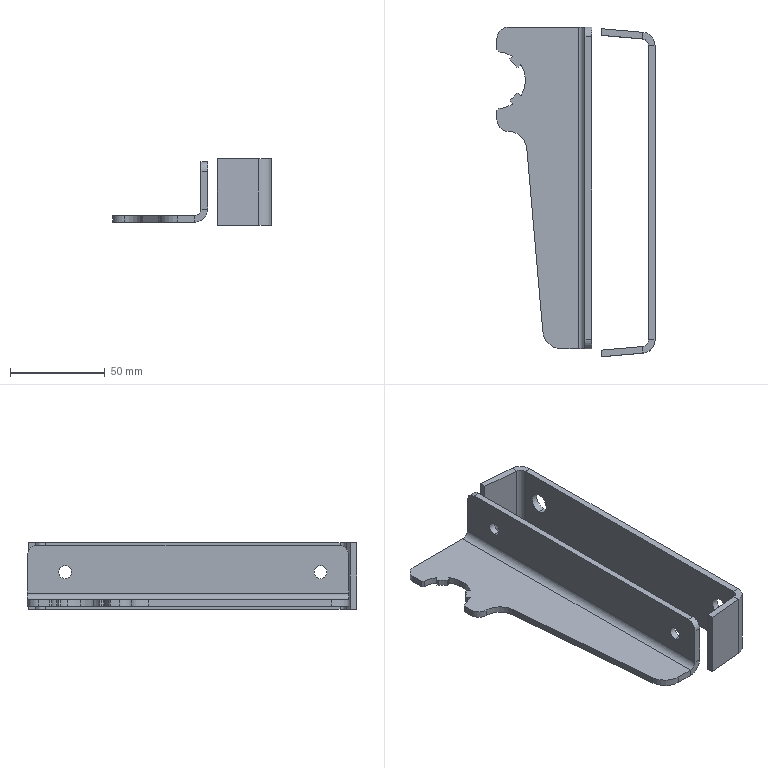Part | STEP file | Symmetry ITEM SUPPORT | 2 solids | 74 faces | box 83.5 x 174.166 x 35 mm | volume 61549 mm3 | plane 42 | cylinder 32 | commonest cylinder face diameters 0.4 x6 6.8 x4 10.5 x4 30 x4 7 x3 14 x3